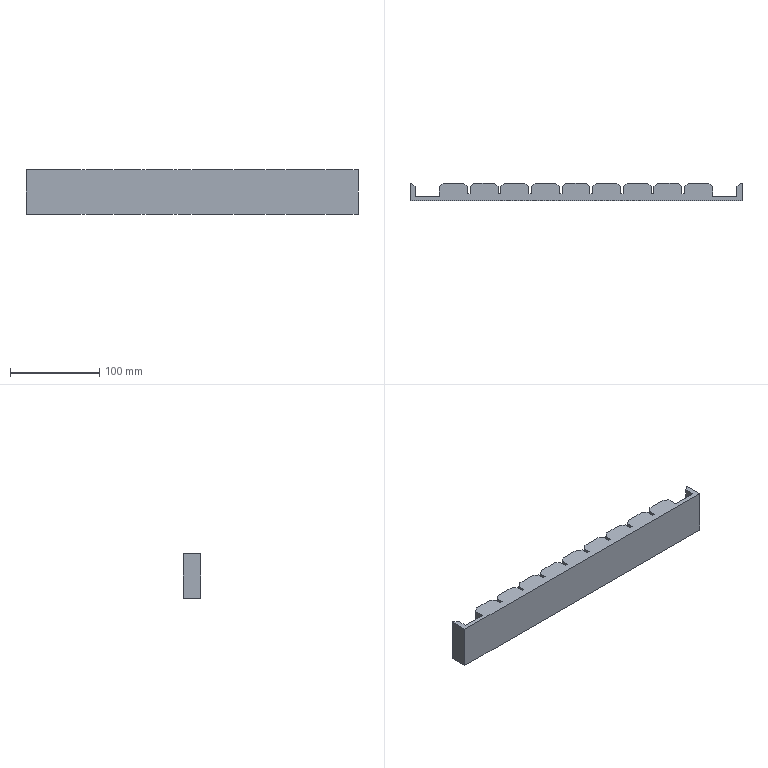NC program | NX | posted with a generic post | part box 372.9 x 20 x 50 mm
Lines 1464 to 3956 of 3956, first 2432 of 2489 lines:
(PLANAR_MILL , TOOL : D3)
N2926 T16 M6
N2928 G17 G43 G0 G90 X-120.54 Y-28. Z30. S9500 H16 M3
N2930 Z2.7
N2932 G94 G1 Z-0.3 F1800.
N2934 Y-25.
N2936 Y25.
N2938 Y28.
N2940 Z2.7
N2942 G0 Y-28. Z2.4
N2944 G1 Z-0.6
N2946 Y-25.
N2948 Y25.
N2950 Y28.
N2952 Z2.4
N2954 G0 Y-28. Z2.1
N2956 G1 Z-0.9
N2958 Y-25.
N2960 Y25.
N2962 Y28.
N2964 Z2.1
N2966 G0 Y-28. Z1.8
N2968 G1 Z-1.2
N2970 Y-25.
N2972 Y25.
N2974 Y28.
N2976 Z1.8
N2978 G0 Y-28. Z1.5
N2980 G1 Z-1.5
N2982 Y-25.
N2984 Y25.
N2986 Y28.
N2988 Z1.5
N2990 G0 Y-28. Z1.2
N2992 G1 Z-1.8
N2994 Y-25.
N2996 Y25.
N2998 Y28.
N3000 Z1.2
N3002 G0 Y-28. Z0.9
N3004 G1 Z-2.1
N3006 Y-25.
N3008 Y25.
N3010 Y28.
N3012 Z0.9
N3014 G0 Y-28. Z0.6
N3016 G1 Z-2.4
N3018 Y-25.
N3020 Y25.
N3022 Y28.
N3024 Z0.6
N3026 G0 Y-28. Z0.3
N3028 G1 Z-2.7
N3030 Y-25.
N3032 Y25.
N3034 Y28.
N3036 Z0.3
N3038 G0 Y-28. Z0.
N3040 G1 Z-3.
N3042 Y-25.
N3044 Y25.
N3046 Y28.
N3048 Z0.
N3050 G0 Y-28. Z-0.3
N3052 G1 Z-3.3
N3054 Y-25.
N3056 Y25.
N3058 Y28.
N3060 Z-0.3
N3062 G0 Y-28. Z-0.6
N3064 G1 Z-3.6
N3066 Y-25.
N3068 Y25.
N3070 Y28.
N3072 Z-0.6
N3074 G0 Y-28. Z-0.9
N3076 G1 Z-3.9
N3078 Y-25.
N3080 Y25.
N3082 Y28.
N3084 Z-0.9
N3086 G0 Y-28. Z-1.2
N3088 G1 Z-4.2
N3090 Y-25.
N3092 Y25.
N3094 Y28.
N3096 Z-1.2
N3098 G0 Y-28. Z-1.5
N3100 G1 Z-4.5
N3102 Y-25.
N3104 Y25.
N3106 Y28.
N3108 Z-1.5
N3110 G0 Y-28. Z-1.8
N3112 G1 Z-4.8
N3114 Y-25.
N3116 Y25.
N3118 Y28.
N3120 Z-1.8
N3122 G0 Y-28. Z-2.1
N3124 G1 Z-5.1
N3126 Y-25.
N3128 Y25.
N3130 Y28.
N3132 Z-2.1
N3134 G0 Y-28. Z-2.4
N3136 G1 Z-5.4
N3138 Y-25.
N3140 Y25.
N3142 Y28.
N3144 Z-2.4
N3146 G0 Y-28. Z-2.7
N3148 G1 Z-5.7
N3150 Y-25.
N3152 Y25.
N3154 Y28.
N3156 Z-2.7
N3158 G0 Y-28. Z-3.
N3160 G1 Z-6.
N3162 Y-25.
N3164 Y25.
N3166 Y28.
N3168 Z-3.
N3170 G0 Y-28. Z-3.3
N3172 G1 Z-6.3
N3174 Y-25.
N3176 Y25.
N3178 Y28.
N3180 Z-3.3
N3182 G0 Y-28. Z-3.6
N3184 G1 Z-6.6
N3186 Y-25.
N3188 Y25.
N3190 Y28.
N3192 Z-3.6
N3194 G0 Y-28. Z-3.9
N3196 G1 Z-6.9
N3198 Y-25.
N3200 Y25.
N3202 Y28.
N3204 Z-3.9
N3206 G0 Y-28. Z-4.2
N3208 G1 Z-7.2
N3210 Y-25.
N3212 Y25.
N3214 Y28.
N3216 Z-4.2
N3218 G0 Y-28. Z-4.5
N3220 G1 Z-7.5
N3222 Y-25.
N3224 Y25.
N3226 Y28.
N3228 Z-4.5
N3230 G0 Y-28. Z-4.8
N3232 G1 Z-7.8
N3234 Y-25.
N3236 Y25.
N3238 Y28.
N3240 Z-4.8
N3242 G0 Y-28. Z-5.1
N3244 G1 Z-8.1
N3246 Y-25.
N3248 Y25.
N3250 Y28.
N3252 Z-5.1
N3254 G0 Y-28. Z-5.4
N3256 G1 Z-8.4
N3258 Y-25.
N3260 Y25.
N3262 Y28.
N3264 Z-5.4
N3266 G0 Y-28. Z-5.7
N3268 G1 Z-8.7
N3270 Y-25.
N3272 Y25.
N3274 Y28.
N3276 Z-5.7
N3278 G0 Y-28. Z-6.
N3280 G1 Z-9.
N3282 Y-25.
N3284 Y25.
N3286 Y28.
N3288 Z-6.
N3290 G0 Y-28. Z-6.3
N3292 G1 Z-9.3
N3294 Y-25.
N3296 Y25.
N3298 Y28.
N3300 Z-6.3
N3302 G0 Y-28. Z-6.6
N3304 G1 Z-9.6
N3306 Y-25.
N3308 Y25.
N3310 Y28.
N3312 Z-6.6
N3314 G0 Y-28. Z-6.9
N3316 G1 Z-9.9
N3318 Y-25.
N3320 Y25.
N3322 Y28.
N3324 Z-6.9
N3326 G0 Y-28. Z-7.2
N3328 G1 Z-10.2
N3330 Y-25.
N3332 Y25.
N3334 Y28.
N3336 Z-7.2
N3338 G0 Y-28. Z-7.5
N3340 G1 Z-10.5
N3342 Y-25.
N3344 Y25.
N3346 Y28.
N3348 Z-7.5
N3350 G0 Y-28. Z-7.8
N3352 G1 Z-10.8
N3354 Y-25.
N3356 Y25.
N3358 Y28.
N3360 Z-7.8
N3362 G0 Y-28. Z-8.1
N3364 G1 Z-11.1
N3366 Y-25.
N3368 Y25.
N3370 Y28.
N3372 Z-8.1
N3374 G0 Y-28. Z-8.4
N3376 G1 Z-11.4
N3378 Y-25.
N3380 Y25.
N3382 Y28.
N3384 Z-8.4
N3386 G0 Y-28. Z-8.7
N3388 G1 Z-11.7
N3390 Y-25.
N3392 Y25.
N3394 Y28.
N3396 Z-8.7
N3398 G0 Y-28. Z-9.
N3400 G1 Z-12.
N3402 Y-25.
N3404 Y25.
N3406 Y28.
N3408 Z-9.
N3410 G0 Z30.
N3412 X-86.1 Y-28.
N3414 Z2.7
N3416 G1 Z-0.3
N3418 Y-25.
N3420 Y25.
N3422 Y28.
N3424 Z2.7
N3426 G0 Y-28. Z2.4
N3428 G1 Z-0.6
N3430 Y-25.
N3432 Y25.
N3434 Y28.
N3436 Z2.4
N3438 G0 Y-28. Z2.1
N3440 G1 Z-0.9
N3442 Y-25.
N3444 Y25.
N3446 Y28.
N3448 Z2.1
N3450 G0 Y-28. Z1.8
N3452 G1 Z-1.2
N3454 Y-25.
N3456 Y25.
N3458 Y28.
N3460 Z1.8
N3462 G0 Y-28. Z1.5
N3464 G1 Z-1.5
N3466 Y-25.
N3468 Y25.
N3470 Y28.
N3472 Z1.5
N3474 G0 Y-28. Z1.2
N3476 G1 Z-1.8
N3478 Y-25.
N3480 Y25.
N3482 Y28.
N3484 Z1.2
N3486 G0 Y-28. Z0.9
N3488 G1 Z-2.1
N3490 Y-25.
N3492 Y25.
N3494 Y28.
N3496 Z0.9
N3498 G0 Y-28. Z0.6
N3500 G1 Z-2.4
N3502 Y-25.
N3504 Y25.
N3506 Y28.
N3508 Z0.6
N3510 G0 Y-28. Z0.3
N3512 G1 Z-2.7
N3514 Y-25.
N3516 Y25.
N3518 Y28.
N3520 Z0.3
N3522 G0 Y-28. Z0.
N3524 G1 Z-3.
N3526 Y-25.
N3528 Y25.
N3530 Y28.
N3532 Z0.
N3534 G0 Y-28. Z-0.3
N3536 G1 Z-3.3
N3538 Y-25.
N3540 Y25.
N3542 Y28.
N3544 Z-0.3
N3546 G0 Y-28. Z-0.6
N3548 G1 Z-3.6
N3550 Y-25.
N3552 Y25.
N3554 Y28.
N3556 Z-0.6
N3558 G0 Y-28. Z-0.9
N3560 G1 Z-3.9
N3562 Y-25.
N3564 Y25.
N3566 Y28.
N3568 Z-0.9
N3570 G0 Y-28. Z-1.2
N3572 G1 Z-4.2
N3574 Y-25.
N3576 Y25.
N3578 Y28.
N3580 Z-1.2
N3582 G0 Y-28. Z-1.5
N3584 G1 Z-4.5
N3586 Y-25.
N3588 Y25.
N3590 Y28.
N3592 Z-1.5
N3594 G0 Y-28. Z-1.8
N3596 G1 Z-4.8
N3598 Y-25.
N3600 Y25.
N3602 Y28.
N3604 Z-1.8
N3606 G0 Y-28. Z-2.1
N3608 G1 Z-5.1
N3610 Y-25.
N3612 Y25.
N3614 Y28.
N3616 Z-2.1
N3618 G0 Y-28. Z-2.4
N3620 G1 Z-5.4
N3622 Y-25.
N3624 Y25.
N3626 Y28.
N3628 Z-2.4
N3630 G0 Y-28. Z-2.7
N3632 G1 Z-5.7
N3634 Y-25.
N3636 Y25.
N3638 Y28.
N3640 Z-2.7
N3642 G0 Y-28. Z-3.
N3644 G1 Z-6.
N3646 Y-25.
N3648 Y25.
N3650 Y28.
N3652 Z-3.
N3654 G0 Y-28. Z-3.3
N3656 G1 Z-6.3
N3658 Y-25.
N3660 Y25.
N3662 Y28.
N3664 Z-3.3
N3666 G0 Y-28. Z-3.6
N3668 G1 Z-6.6
N3670 Y-25.
N3672 Y25.
N3674 Y28.
N3676 Z-3.6
N3678 G0 Y-28. Z-3.9
N3680 G1 Z-6.9
N3682 Y-25.
N3684 Y25.
N3686 Y28.
N3688 Z-3.9
N3690 G0 Y-28. Z-4.2
N3692 G1 Z-7.2
N3694 Y-25.
N3696 Y25.
N3698 Y28.
N3700 Z-4.2
N3702 G0 Y-28. Z-4.5
N3704 G1 Z-7.5
N3706 Y-25.
N3708 Y25.
N3710 Y28.
N3712 Z-4.5
N3714 G0 Y-28. Z-4.8
N3716 G1 Z-7.8
N3718 Y-25.
N3720 Y25.
N3722 Y28.
N3724 Z-4.8
N3726 G0 Y-28. Z-5.1
N3728 G1 Z-8.1
N3730 Y-25.
N3732 Y25.
N3734 Y28.
N3736 Z-5.1
N3738 G0 Y-28. Z-5.4
N3740 G1 Z-8.4
N3742 Y-25.
N3744 Y25.
N3746 Y28.
N3748 Z-5.4
N3750 G0 Y-28. Z-5.7
N3752 G1 Z-8.7
N3754 Y-25.
N3756 Y25.
N3758 Y28.
N3760 Z-5.7
N3762 G0 Y-28. Z-6.
N3764 G1 Z-9.
N3766 Y-25.
N3768 Y25.
N3770 Y28.
N3772 Z-6.
N3774 G0 Y-28. Z-6.3
N3776 G1 Z-9.3
N3778 Y-25.
N3780 Y25.
N3782 Y28.
N3784 Z-6.3
N3786 G0 Y-28. Z-6.6
N3788 G1 Z-9.6
N3790 Y-25.
N3792 Y25.
N3794 Y28.
N3796 Z-6.6
N3798 G0 Y-28. Z-6.9
N3800 G1 Z-9.9
N3802 Y-25.
N3804 Y25.
N3806 Y28.
N3808 Z-6.9
N3810 G0 Y-28. Z-7.2
N3812 G1 Z-10.2
N3814 Y-25.
N3816 Y25.
N3818 Y28.
N3820 Z-7.2
N3822 G0 Y-28. Z-7.5
N3824 G1 Z-10.5
N3826 Y-25.
N3828 Y25.
N3830 Y28.
N3832 Z-7.5
N3834 G0 Y-28. Z-7.8
N3836 G1 Z-10.8
N3838 Y-25.
N3840 Y25.
N3842 Y28.
N3844 Z-7.8
N3846 G0 Y-28. Z-8.1
N3848 G1 Z-11.1
N3850 Y-25.
N3852 Y25.
N3854 Y28.
N3856 Z-8.1
N3858 G0 Y-28. Z-8.4
N3860 G1 Z-11.4
N3862 Y-25.
N3864 Y25.
N3866 Y28.
N3868 Z-8.4
N3870 G0 Y-28. Z-8.7
N3872 G1 Z-11.7
N3874 Y-25.
N3876 Y25.
N3878 Y28.
N3880 Z-8.7
N3882 G0 Y-28. Z-9.
N3884 G1 Z-12.
N3886 Y-25.
N3888 Y25.
N3890 Y28.
N3892 Z-9.
N3894 G0 Z30.
N3896 X-51.66 Y-28.
N3898 Z2.7
N3900 G1 Z-0.3
N3902 Y-25.
N3904 Y25.
N3906 Y28.
N3908 Z2.7
N3910 G0 Y-28. Z2.4
N3912 G1 Z-0.6
N3914 Y-25.
N3916 Y25.
N3918 Y28.
N3920 Z2.4
N3922 G0 Y-28. Z2.1
N3924 G1 Z-0.9
N3926 Y-25.
N3928 Y25.
N3930 Y28.
N3932 Z2.1
N3934 G0 Y-28. Z1.8
N3936 G1 Z-1.2
N3938 Y-25.
N3940 Y25.
N3942 Y28.
N3944 Z1.8
N3946 G0 Y-28. Z1.5
N3948 G1 Z-1.5
N3950 Y-25.
N3952 Y25.
N3954 Y28.
N3956 Z1.5
N3958 G0 Y-28. Z1.2
N3960 G1 Z-1.8
N3962 Y-25.
N3964 Y25.
N3966 Y28.
N3968 Z1.2
N3970 G0 Y-28. Z0.9
N3972 G1 Z-2.1
N3974 Y-25.
N3976 Y25.
N3978 Y28.
N3980 Z0.9
N3982 G0 Y-28. Z0.6
N3984 G1 Z-2.4
N3986 Y-25.
N3988 Y25.
N3990 Y28.
N3992 Z0.6
N3994 G0 Y-28. Z0.3
N3996 G1 Z-2.7
N3998 Y-25.
N4000 Y25.
N4002 Y28.
N4004 Z0.3
N4006 G0 Y-28. Z0.
N4008 G1 Z-3.
N4010 Y-25.
N4012 Y25.
N4014 Y28.
N4016 Z0.
N4018 G0 Y-28. Z-0.3
N4020 G1 Z-3.3
N4022 Y-25.
N4024 Y25.
N4026 Y28.
N4028 Z-0.3
N4030 G0 Y-28. Z-0.6
N4032 G1 Z-3.6
N4034 Y-25.
N4036 Y25.
N4038 Y28.
N4040 Z-0.6
N4042 G0 Y-28. Z-0.9
N4044 G1 Z-3.9
N4046 Y-25.
N4048 Y25.
N4050 Y28.
N4052 Z-0.9
N4054 G0 Y-28. Z-1.2
N4056 G1 Z-4.2
N4058 Y-25.
N4060 Y25.
N4062 Y28.
N4064 Z-1.2
N4066 G0 Y-28. Z-1.5
N4068 G1 Z-4.5
N4070 Y-25.
N4072 Y25.
N4074 Y28.
N4076 Z-1.5
N4078 G0 Y-28. Z-1.8
N4080 G1 Z-4.8
N4082 Y-25.
N4084 Y25.
N4086 Y28.
N4088 Z-1.8
N4090 G0 Y-28. Z-2.1
N4092 G1 Z-5.1
N4094 Y-25.
N4096 Y25.
N4098 Y28.
N4100 Z-2.1
N4102 G0 Y-28. Z-2.4
N4104 G1 Z-5.4
N4106 Y-25.
N4108 Y25.
N4110 Y28.
N4112 Z-2.4
N4114 G0 Y-28. Z-2.7
N4116 G1 Z-5.7
N4118 Y-25.
N4120 Y25.
N4122 Y28.
N4124 Z-2.7
N4126 G0 Y-28. Z-3.
N4128 G1 Z-6.
N4130 Y-25.
N4132 Y25.
N4134 Y28.
N4136 Z-3.
N4138 G0 Y-28. Z-3.3
N4140 G1 Z-6.3
N4142 Y-25.
N4144 Y25.
N4146 Y28.
N4148 Z-3.3
N4150 G0 Y-28. Z-3.6
N4152 G1 Z-6.6
N4154 Y-25.
N4156 Y25.
N4158 Y28.
N4160 Z-3.6
N4162 G0 Y-28. Z-3.9
N4164 G1 Z-6.9
N4166 Y-25.
N4168 Y25.
N4170 Y28.
N4172 Z-3.9
N4174 G0 Y-28. Z-4.2
N4176 G1 Z-7.2
N4178 Y-25.
N4180 Y25.
N4182 Y28.
N4184 Z-4.2
N4186 G0 Y-28. Z-4.5
N4188 G1 Z-7.5
N4190 Y-25.
N4192 Y25.
N4194 Y28.
N4196 Z-4.5
N4198 G0 Y-28. Z-4.8
N4200 G1 Z-7.8
N4202 Y-25.
N4204 Y25.
N4206 Y28.
N4208 Z-4.8
N4210 G0 Y-28. Z-5.1
N4212 G1 Z-8.1
N4214 Y-25.
N4216 Y25.
N4218 Y28.
N4220 Z-5.1
N4222 G0 Y-28. Z-5.4
N4224 G1 Z-8.4
N4226 Y-25.
N4228 Y25.
N4230 Y28.
N4232 Z-5.4
N4234 G0 Y-28. Z-5.7
N4236 G1 Z-8.7
N4238 Y-25.
N4240 Y25.
N4242 Y28.
N4244 Z-5.7
N4246 G0 Y-28. Z-6.
N4248 G1 Z-9.
N4250 Y-25.
N4252 Y25.
N4254 Y28.
N4256 Z-6.
N4258 G0 Y-28. Z-6.3
N4260 G1 Z-9.3
N4262 Y-25.
N4264 Y25.
N4266 Y28.
N4268 Z-6.3
N4270 G0 Y-28. Z-6.6
N4272 G1 Z-9.6
N4274 Y-25.
N4276 Y25.
N4278 Y28.
N4280 Z-6.6
N4282 G0 Y-28. Z-6.9
N4284 G1 Z-9.9
N4286 Y-25.
N4288 Y25.
N4290 Y28.
N4292 Z-6.9
N4294 G0 Y-28. Z-7.2
N4296 G1 Z-10.2
N4298 Y-25.
N4300 Y25.
N4302 Y28.
N4304 Z-7.2
N4306 G0 Y-28. Z-7.5
N4308 G1 Z-10.5
N4310 Y-25.
N4312 Y25.
N4314 Y28.
N4316 Z-7.5
N4318 G0 Y-28. Z-7.8
N4320 G1 Z-10.8
N4322 Y-25.
N4324 Y25.
N4326 Y28.
N4328 Z-7.8
N4330 G0 Y-28. Z-8.1
N4332 G1 Z-11.1
N4334 Y-25.
N4336 Y25.
N4338 Y28.
N4340 Z-8.1
N4342 G0 Y-28. Z-8.4
N4344 G1 Z-11.4
N4346 Y-25.
N4348 Y25.
N4350 Y28.
N4352 Z-8.4
N4354 G0 Y-28. Z-8.7
N4356 G1 Z-11.7
N4358 Y-25.
N4360 Y25.
N4362 Y28.
N4364 Z-8.7
N4366 G0 Y-28. Z-9.
N4368 G1 Z-12.
N4370 Y-25.
N4372 Y25.
N4374 Y28.
N4376 Z-9.
N4378 G0 Z30.
N4380 X-17.22 Y-28.
N4382 Z2.7
N4384 G1 Z-0.3
N4386 Y-25.
N4388 Y25.
N4390 Y28.
N4392 Z2.7
N4394 G0 Y-28. Z2.4
N4396 G1 Z-0.6
N4398 Y-25.
N4400 Y25.
N4402 Y28.
N4404 Z2.4
N4406 G0 Y-28. Z2.1
N4408 G1 Z-0.9
N4410 Y-25.
N4412 Y25.
N4414 Y28.
N4416 Z2.1
N4418 G0 Y-28. Z1.8
N4420 G1 Z-1.2
N4422 Y-25.
N4424 Y25.
N4426 Y28.
N4428 Z1.8
N4430 G0 Y-28. Z1.5
N4432 G1 Z-1.5
N4434 Y-25.
N4436 Y25.
N4438 Y28.
N4440 Z1.5
N4442 G0 Y-28. Z1.2
N4444 G1 Z-1.8
N4446 Y-25.
N4448 Y25.
N4450 Y28.
N4452 Z1.2
N4454 G0 Y-28. Z0.9
N4456 G1 Z-2.1
N4458 Y-25.
N4460 Y25.
N4462 Y28.
N4464 Z0.9
N4466 G0 Y-28. Z0.6
N4468 G1 Z-2.4
N4470 Y-25.
N4472 Y25.
N4474 Y28.
N4476 Z0.6
N4478 G0 Y-28. Z0.3
N4480 G1 Z-2.7
N4482 Y-25.
N4484 Y25.
N4486 Y28.
N4488 Z0.3
N4490 G0 Y-28. Z0.
N4492 G1 Z-3.
N4494 Y-25.
N4496 Y25.
N4498 Y28.
N4500 Z0.
N4502 G0 Y-28. Z-0.3
N4504 G1 Z-3.3
N4506 Y-25.
N4508 Y25.
N4510 Y28.
N4512 Z-0.3
N4514 G0 Y-28. Z-0.6
N4516 G1 Z-3.6
N4518 Y-25.
N4520 Y25.
N4522 Y28.
N4524 Z-0.6
N4526 G0 Y-28. Z-0.9
N4528 G1 Z-3.9
N4530 Y-25.
N4532 Y25.
N4534 Y28.
N4536 Z-0.9
N4538 G0 Y-28. Z-1.2
N4540 G1 Z-4.2
N4542 Y-25.
N4544 Y25.
N4546 Y28.
N4548 Z-1.2
N4550 G0 Y-28. Z-1.5
N4552 G1 Z-4.5
N4554 Y-25.
N4556 Y25.
N4558 Y28.
N4560 Z-1.5
N4562 G0 Y-28. Z-1.8
N4564 G1 Z-4.8
N4566 Y-25.
N4568 Y25.
N4570 Y28.
N4572 Z-1.8
N4574 G0 Y-28. Z-2.1
N4576 G1 Z-5.1
N4578 Y-25.
N4580 Y25.
N4582 Y28.
N4584 Z-2.1
N4586 G0 Y-28. Z-2.4
N4588 G1 Z-5.4
N4590 Y-25.
N4592 Y25.
N4594 Y28.
N4596 Z-2.4
N4598 G0 Y-28. Z-2.7
N4600 G1 Z-5.7
N4602 Y-25.
N4604 Y25.
N4606 Y28.
N4608 Z-2.7
N4610 G0 Y-28. Z-3.
N4612 G1 Z-6.
N4614 Y-25.
N4616 Y25.
N4618 Y28.
N4620 Z-3.
N4622 G0 Y-28. Z-3.3
N4624 G1 Z-6.3
N4626 Y-25.
N4628 Y25.
N4630 Y28.
N4632 Z-3.3
N4634 G0 Y-28. Z-3.6
N4636 G1 Z-6.6
N4638 Y-25.
N4640 Y25.
N4642 Y28.
N4644 Z-3.6
N4646 G0 Y-28. Z-3.9
N4648 G1 Z-6.9
N4650 Y-25.
N4652 Y25.
N4654 Y28.
N4656 Z-3.9
N4658 G0 Y-28. Z-4.2
N4660 G1 Z-7.2
N4662 Y-25.
N4664 Y25.
N4666 Y28.
N4668 Z-4.2
N4670 G0 Y-28. Z-4.5
N4672 G1 Z-7.5
N4674 Y-25.
N4676 Y25.
N4678 Y28.
N4680 Z-4.5
N4682 G0 Y-28. Z-4.8
N4684 G1 Z-7.8
N4686 Y-25.
N4688 Y25.
N4690 Y28.
N4692 Z-4.8
N4694 G0 Y-28. Z-5.1
N4696 G1 Z-8.1
N4698 Y-25.
N4700 Y25.
N4702 Y28.
N4704 Z-5.1
N4706 G0 Y-28. Z-5.4
N4708 G1 Z-8.4
N4710 Y-25.
N4712 Y25.
N4714 Y28.
N4716 Z-5.4
N4718 G0 Y-28. Z-5.7
N4720 G1 Z-8.7
N4722 Y-25.
N4724 Y25.
N4726 Y28.
N4728 Z-5.7
N4730 G0 Y-28. Z-6.
N4732 G1 Z-9.
N4734 Y-25.
N4736 Y25.
N4738 Y28.
N4740 Z-6.
N4742 G0 Y-28. Z-6.3
N4744 G1 Z-9.3
N4746 Y-25.
N4748 Y25.
N4750 Y28.
N4752 Z-6.3
N4754 G0 Y-28. Z-6.6
N4756 G1 Z-9.6
N4758 Y-25.
N4760 Y25.
N4762 Y28.
N4764 Z-6.6
N4766 G0 Y-28. Z-6.9
N4768 G1 Z-9.9
N4770 Y-25.
N4772 Y25.
N4774 Y28.
N4776 Z-6.9
N4778 G0 Y-28. Z-7.2
N4780 G1 Z-10.2
N4782 Y-25.
N4784 Y25.
N4786 Y28.
N4788 Z-7.2
N4790 G0 Y-28. Z-7.5
N4792 G1 Z-10.5
N4794 Y-25.
N4796 Y25.
N4798 Y28.
N4800 Z-7.5
N4802 G0 Y-28. Z-7.8
N4804 G1 Z-10.8
N4806 Y-25.
N4808 Y25.
N4810 Y28.
N4812 Z-7.8
N4814 G0 Y-28. Z-8.1
N4816 G1 Z-11.1
N4818 Y-25.
N4820 Y25.
N4822 Y28.
N4824 Z-8.1
N4826 G0 Y-28. Z-8.4
N4828 G1 Z-11.4
N4830 Y-25.
N4832 Y25.
N4834 Y28.
N4836 Z-8.4
N4838 G0 Y-28. Z-8.7
N4840 G1 Z-11.7
N4842 Y-25.
N4844 Y25.
N4846 Y28.
N4848 Z-8.7
N4850 G0 Y-28. Z-9.
N4852 G1 Z-12.
N4854 Y-25.
N4856 Y25.
N4858 Y28.
N4860 Z-9.
N4862 G0 Z30.
N4864 X17.22 Y-28.
N4866 Z2.7
N4868 G1 Z-0.3
N4870 Y-25.
N4872 Y25.
N4874 Y28.
N4876 Z2.7
N4878 G0 Y-28. Z2.4
N4880 G1 Z-0.6
N4882 Y-25.
N4884 Y25.
N4886 Y28.
N4888 Z2.4
N4890 G0 Y-28. Z2.1
N4892 G1 Z-0.9
N4894 Y-25.
N4896 Y25.
N4898 Y28.
N4900 Z2.1
N4902 G0 Y-28. Z1.8
N4904 G1 Z-1.2
N4906 Y-25.
N4908 Y25.
N4910 Y28.
N4912 Z1.8
N4914 G0 Y-28. Z1.5
N4916 G1 Z-1.5
N4918 Y-25.
N4920 Y25.
N4922 Y28.
N4924 Z1.5
N4926 G0 Y-28. Z1.2
N4928 G1 Z-1.8
N4930 Y-25.
N4932 Y25.
N4934 Y28.
N4936 Z1.2
N4938 G0 Y-28. Z0.9
N4940 G1 Z-2.1
N4942 Y-25.
N4944 Y25.
N4946 Y28.
N4948 Z0.9
N4950 G0 Y-28. Z0.6
N4952 G1 Z-2.4
N4954 Y-25.
N4956 Y25.
N4958 Y28.
N4960 Z0.6
N4962 G0 Y-28. Z0.3
N4964 G1 Z-2.7
N4966 Y-25.
N4968 Y25.
N4970 Y28.
N4972 Z0.3
N4974 G0 Y-28. Z0.
N4976 G1 Z-3.
N4978 Y-25.
N4980 Y25.
N4982 Y28.
N4984 Z0.
N4986 G0 Y-28. Z-0.3
N4988 G1 Z-3.3
N4990 Y-25.
N4992 Y25.
N4994 Y28.
N4996 Z-0.3
N4998 G0 Y-28. Z-0.6
N5000 G1 Z-3.6
N5002 Y-25.
N5004 Y25.
N5006 Y28.
N5008 Z-0.6
N5010 G0 Y-28. Z-0.9
N5012 G1 Z-3.9
N5014 Y-25.
N5016 Y25.
N5018 Y28.
N5020 Z-0.9
N5022 G0 Y-28. Z-1.2
N5024 G1 Z-4.2
N5026 Y-25.
N5028 Y25.
N5030 Y28.
N5032 Z-1.2
N5034 G0 Y-28. Z-1.5
N5036 G1 Z-4.5
N5038 Y-25.
N5040 Y25.
N5042 Y28.
N5044 Z-1.5
N5046 G0 Y-28. Z-1.8
N5048 G1 Z-4.8
N5050 Y-25.
N5052 Y25.
N5054 Y28.
N5056 Z-1.8
N5058 G0 Y-28. Z-2.1
N5060 G1 Z-5.1
N5062 Y-25.
N5064 Y25.
N5066 Y28.
N5068 Z-2.1
N5070 G0 Y-28. Z-2.4
N5072 G1 Z-5.4
N5074 Y-25.
N5076 Y25.
N5078 Y28.
N5080 Z-2.4
N5082 G0 Y-28. Z-2.7
N5084 G1 Z-5.7
N5086 Y-25.
N5088 Y25.
N5090 Y28.
N5092 Z-2.7
N5094 G0 Y-28. Z-3.
N5096 G1 Z-6.
N5098 Y-25.
N5100 Y25.
N5102 Y28.
N5104 Z-3.
N5106 G0 Y-28. Z-3.3
N5108 G1 Z-6.3
N5110 Y-25.
N5112 Y25.
N5114 Y28.
N5116 Z-3.3
N5118 G0 Y-28. Z-3.6
N5120 G1 Z-6.6
N5122 Y-25.
N5124 Y25.
N5126 Y28.
N5128 Z-3.6
N5130 G0 Y-28. Z-3.9
N5132 G1 Z-6.9
N5134 Y-25.
N5136 Y25.
N5138 Y28.
N5140 Z-3.9
N5142 G0 Y-28. Z-4.2
N5144 G1 Z-7.2
N5146 Y-25.
N5148 Y25.
N5150 Y28.
N5152 Z-4.2
N5154 G0 Y-28. Z-4.5
N5156 G1 Z-7.5
N5158 Y-25.
N5160 Y25.
N5162 Y28.
N5164 Z-4.5
N5166 G0 Y-28. Z-4.8
N5168 G1 Z-7.8
N5170 Y-25.
N5172 Y25.
N5174 Y28.
N5176 Z-4.8
N5178 G0 Y-28. Z-5.1
N5180 G1 Z-8.1
N5182 Y-25.
N5184 Y25.
N5186 Y28.
N5188 Z-5.1
N5190 G0 Y-28. Z-5.4
N5192 G1 Z-8.4
N5194 Y-25.
N5196 Y25.
N5198 Y28.
N5200 Z-5.4
N5202 G0 Y-28. Z-5.7
N5204 G1 Z-8.7
N5206 Y-25.
N5208 Y25.
N5210 Y28.
N5212 Z-5.7
N5214 G0 Y-28. Z-6.
N5216 G1 Z-9.
N5218 Y-25.
N5220 Y25.
N5222 Y28.
N5224 Z-6.
N5226 G0 Y-28. Z-6.3
N5228 G1 Z-9.3
N5230 Y-25.
N5232 Y25.
N5234 Y28.
N5236 Z-6.3
N5238 G0 Y-28. Z-6.6
N5240 G1 Z-9.6
N5242 Y-25.
N5244 Y25.
N5246 Y28.
N5248 Z-6.6
N5250 G0 Y-28. Z-6.9
N5252 G1 Z-9.9
N5254 Y-25.
N5256 Y25.
N5258 Y28.
N5260 Z-6.9
N5262 G0 Y-28. Z-7.2
N5264 G1 Z-10.2
N5266 Y-25.
N5268 Y25.
N5270 Y28.
N5272 Z-7.2
N5274 G0 Y-28. Z-7.5
N5276 G1 Z-10.5
N5278 Y-25.
N5280 Y25.
N5282 Y28.
N5284 Z-7.5
N5286 G0 Y-28. Z-7.8
N5288 G1 Z-10.8
N5290 Y-25.
N5292 Y25.
N5294 Y28.
N5296 Z-7.8
N5298 G0 Y-28. Z-8.1
N5300 G1 Z-11.1
N5302 Y-25.
N5304 Y25.
N5306 Y28.
N5308 Z-8.1
N5310 G0 Y-28. Z-8.4
N5312 G1 Z-11.4
N5314 Y-25.
N5316 Y25.
N5318 Y28.
N5320 Z-8.4
N5322 G0 Y-28. Z-8.7
N5324 G1 Z-11.7
N5326 Y-25.
N5328 Y25.
N5330 Y28.
N5332 Z-8.7
N5334 G0 Y-28. Z-9.
N5336 G1 Z-12.
N5338 Y-25.
N5340 Y25.
N5342 Y28.
N5344 Z-9.
N5346 G0 Z30.
N5348 X51.66 Y-28.
N5350 Z2.7
N5352 G1 Z-0.3
N5354 Y-25.
N5356 Y25.
N5358 Y28.
N5360 Z2.7
N5362 G0 Y-28. Z2.4
N5364 G1 Z-0.6
N5366 Y-25.
N5368 Y25.
N5370 Y28.
N5372 Z2.4
N5374 G0 Y-28. Z2.1
N5376 G1 Z-0.9
N5378 Y-25.
N5380 Y25.
N5382 Y28.
N5384 Z2.1
N5386 G0 Y-28. Z1.8
N5388 G1 Z-1.2
N5390 Y-25.
N5392 Y25.
N5394 Y28.
N5396 Z1.8
N5398 G0 Y-28. Z1.5
N5400 G1 Z-1.5
N5402 Y-25.
N5404 Y25.
N5406 Y28.
N5408 Z1.5
N5410 G0 Y-28. Z1.2
N5412 G1 Z-1.8
N5414 Y-25.
N5416 Y25.
N5418 Y28.
N5420 Z1.2
N5422 G0 Y-28. Z0.9
N5424 G1 Z-2.1
N5426 Y-25.
N5428 Y25.
N5430 Y28.
N5432 Z0.9
N5434 G0 Y-28. Z0.6
N5436 G1 Z-2.4
N5438 Y-25.
N5440 Y25.
N5442 Y28.
N5444 Z0.6
N5446 G0 Y-28. Z0.3
N5448 G1 Z-2.7
N5450 Y-25.
N5452 Y25.
N5454 Y28.
N5456 Z0.3
N5458 G0 Y-28. Z0.
N5460 G1 Z-3.
N5462 Y-25.
N5464 Y25.
N5466 Y28.
N5468 Z0.
N5470 G0 Y-28. Z-0.3
N5472 G1 Z-3.3
N5474 Y-25.
N5476 Y25.
N5478 Y28.
N5480 Z-0.3
N5482 G0 Y-28. Z-0.6
N5484 G1 Z-3.6
N5486 Y-25.
N5488 Y25.
N5490 Y28.
N5492 Z-0.6
N5494 G0 Y-28. Z-0.9
N5496 G1 Z-3.9
N5498 Y-25.
N5500 Y25.
N5502 Y28.
N5504 Z-0.9
N5506 G0 Y-28. Z-1.2
N5508 G1 Z-4.2
N5510 Y-25.
N5512 Y25.
N5514 Y28.
N5516 Z-1.2
N5518 G0 Y-28. Z-1.5
N5520 G1 Z-4.5
N5522 Y-25.
N5524 Y25.
N5526 Y28.
N5528 Z-1.5
N5530 G0 Y-28. Z-1.8
N5532 G1 Z-4.8
N5534 Y-25.
N5536 Y25.
N5538 Y28.
N5540 Z-1.8
N5542 G0 Y-28. Z-2.1
N5544 G1 Z-5.1
N5546 Y-25.
N5548 Y25.
N5550 Y28.
N5552 Z-2.1
N5554 G0 Y-28. Z-2.4
N5556 G1 Z-5.4
N5558 Y-25.
N5560 Y25.
N5562 Y28.
N5564 Z-2.4
N5566 G0 Y-28. Z-2.7
N5568 G1 Z-5.7
N5570 Y-25.
N5572 Y25.
N5574 Y28.
N5576 Z-2.7
N5578 G0 Y-28. Z-3.
N5580 G1 Z-6.
N5582 Y-25.
N5584 Y25.
N5586 Y28.
N5588 Z-3.
N5590 G0 Y-28. Z-3.3
N5592 G1 Z-6.3
N5594 Y-25.
N5596 Y25.
N5598 Y28.
N5600 Z-3.3
N5602 G0 Y-28. Z-3.6
N5604 G1 Z-6.6
N5606 Y-25.
N5608 Y25.
N5610 Y28.
N5612 Z-3.6
N5614 G0 Y-28. Z-3.9
N5616 G1 Z-6.9
N5618 Y-25.
N5620 Y25.
N5622 Y28.
N5624 Z-3.9
N5626 G0 Y-28. Z-4.2
N5628 G1 Z-7.2
N5630 Y-25.
N5632 Y25.
N5634 Y28.
N5636 Z-4.2
N5638 G0 Y-28. Z-4.5
N5640 G1 Z-7.5
N5642 Y-25.
N5644 Y25.
N5646 Y28.
N5648 Z-4.5
N5650 G0 Y-28. Z-4.8
N5652 G1 Z-7.8
N5654 Y-25.
N5656 Y25.
N5658 Y28.
N5660 Z-4.8
N5662 G0 Y-28. Z-5.1
N5664 G1 Z-8.1
N5666 Y-25.
N5668 Y25.
N5670 Y28.
N5672 Z-5.1
N5674 G0 Y-28. Z-5.4
N5676 G1 Z-8.4
N5678 Y-25.
N5680 Y25.
N5682 Y28.
N5684 Z-5.4
N5686 G0 Y-28. Z-5.7
N5688 G1 Z-8.7
N5690 Y-25.
N5692 Y25.
N5694 Y28.
N5696 Z-5.7
N5698 G0 Y-28. Z-6.
N5700 G1 Z-9.
N5702 Y-25.
N5704 Y25.
N5706 Y28.
N5708 Z-6.
N5710 G0 Y-28. Z-6.3
N5712 G1 Z-9.3
N5714 Y-25.
N5716 Y25.
N5718 Y28.
N5720 Z-6.3
N5722 G0 Y-28. Z-6.6
N5724 G1 Z-9.6
N5726 Y-25.
N5728 Y25.
N5730 Y28.
N5732 Z-6.6
N5734 G0 Y-28. Z-6.9
N5736 G1 Z-9.9
N5738 Y-25.
N5740 Y25.
N5742 Y28.
N5744 Z-6.9
N5746 G0 Y-28. Z-7.2
N5748 G1 Z-10.2
N5750 Y-25.
N5752 Y25.
N5754 Y28.
N5756 Z-7.2
N5758 G0 Y-28. Z-7.5
N5760 G1 Z-10.5
N5762 Y-25.
N5764 Y25.
N5766 Y28.
N5768 Z-7.5
N5770 G0 Y-28. Z-7.8
N5772 G1 Z-10.8
N5774 Y-25.
N5776 Y25.
N5778 Y28.
N5780 Z-7.8
N5782 G0 Y-28. Z-8.1
N5784 G1 Z-11.1
N5786 Y-25.
N5788 Y25.
N5790 Y28.
N5792 Z-8.1
N5794 G0 Y-28. Z-8.4
N5796 G1 Z-11.4
N5798 Y-25.
N5800 Y25.
N5802 Y28.
N5804 Z-8.4
N5806 G0 Y-28. Z-8.7
N5808 G1 Z-11.7
N5810 Y-25.
N5812 Y25.
N5814 Y28.
N5816 Z-8.7
N5818 G0 Y-28. Z-9.
N5820 G1 Z-12.
N5822 Y-25.
N5824 Y25.
N5826 Y28.
N5828 Z-9.
N5830 G0 Z30.
N5832 X86.1 Y-28.
N5834 Z2.7
N5836 G1 Z-0.3
N5838 Y-25.
N5840 Y25.
N5842 Y28.
N5844 Z2.7
N5846 G0 Y-28. Z2.4
N5848 G1 Z-0.6
N5850 Y-25.
N5852 Y25.
N5854 Y28.
N5856 Z2.4
N5858 G0 Y-28. Z2.1
N5860 G1 Z-0.9
N5862 Y-25.
N5864 Y25.
N5866 Y28.
N5868 Z2.1
N5870 G0 Y-28. Z1.8
N5872 G1 Z-1.2
N5874 Y-25.
N5876 Y25.
N5878 Y28.
N5880 Z1.8
N5882 G0 Y-28. Z1.5
N5884 G1 Z-1.5
N5886 Y-25.
N5888 Y25.
N5890 Y28.
N5892 Z1.5
N5894 G0 Y-28. Z1.2
N5896 G1 Z-1.8
N5898 Y-25.
N5900 Y25.
N5902 Y28.
N5904 Z1.2
N5906 G0 Y-28. Z0.9
N5908 G1 Z-2.1
N5910 Y-25.
N5912 Y25.
N5914 Y28.
N5916 Z0.9
N5918 G0 Y-28. Z0.6
N5920 G1 Z-2.4
N5922 Y-25.
N5924 Y25.
N5926 Y28.
N5928 Z0.6
N5930 G0 Y-28. Z0.3
N5932 G1 Z-2.7
N5934 Y-25.
N5936 Y25.
N5938 Y28.
N5940 Z0.3
N5942 G0 Y-28. Z0.
N5944 G1 Z-3.
N5946 Y-25.
N5948 Y25.
N5950 Y28.
N5952 Z0.
N5954 G0 Y-28. Z-0.3
N5956 G1 Z-3.3
N5958 Y-25.
N5960 Y25.
N5962 Y28.
N5964 Z-0.3
N5966 G0 Y-28. Z-0.6
N5968 G1 Z-3.6
N5970 Y-25.
N5972 Y25.
N5974 Y28.
N5976 Z-0.6
N5978 G0 Y-28. Z-0.9
N5980 G1 Z-3.9
N5982 Y-25.
N5984 Y25.
N5986 Y28.
N5988 Z-0.9
N5990 G0 Y-28. Z-1.2
N5992 G1 Z-4.2
N5994 Y-25.
N5996 Y25.
N5998 Y28.
N6000 Z-1.2
N6002 G0 Y-28. Z-1.5
N6004 G1 Z-4.5
N6006 Y-25.
N6008 Y25.
N6010 Y28.
N6012 Z-1.5
N6014 G0 Y-28. Z-1.8
N6016 G1 Z-4.8
N6018 Y-25.
N6020 Y25.
N6022 Y28.
N6024 Z-1.8
N6026 G0 Y-28. Z-2.1
N6028 G1 Z-5.1
N6030 Y-25.
N6032 Y25.
N6034 Y28.
N6036 Z-2.1
N6038 G0 Y-28. Z-2.4
N6040 G1 Z-5.4
N6042 Y-25.
N6044 Y25.
N6046 Y28.
N6048 Z-2.4
N6050 G0 Y-28. Z-2.7
N6052 G1 Z-5.7
N6054 Y-25.
N6056 Y25.
N6058 Y28.
N6060 Z-2.7
N6062 G0 Y-28. Z-3.
N6064 G1 Z-6.
N6066 Y-25.
N6068 Y25.
N6070 Y28.
N6072 Z-3.
N6074 G0 Y-28. Z-3.3
N6076 G1 Z-6.3
N6078 Y-25.
N6080 Y25.
N6082 Y28.
N6084 Z-3.3
N6086 G0 Y-28. Z-3.6
N6088 G1 Z-6.6
N6090 Y-25.
N6092 Y25.
N6094 Y28.
N6096 Z-3.6
N6098 G0 Y-28. Z-3.9
N6100 G1 Z-6.9
N6102 Y-25.
N6104 Y25.
N6106 Y28.
N6108 Z-3.9
N6110 G0 Y-28. Z-4.2
N6112 G1 Z-7.2
N6114 Y-25.
N6116 Y25.
N6118 Y28.
N6120 Z-4.2
N6122 G0 Y-28. Z-4.5
N6124 G1 Z-7.5
N6126 Y-25.
N6128 Y25.
N6130 Y28.
N6132 Z-4.5
N6134 G0 Y-28. Z-4.8
N6136 G1 Z-7.8
N6138 Y-25.
N6140 Y25.
N6142 Y28.
N6144 Z-4.8
N6146 G0 Y-28. Z-5.1
N6148 G1 Z-8.1
N6150 Y-25.
N6152 Y25.
N6154 Y28.
N6156 Z-5.1
N6158 G0 Y-28. Z-5.4
N6160 G1 Z-8.4
N6162 Y-25.
N6164 Y25.
N6166 Y28.
N6168 Z-5.4
N6170 G0 Y-28. Z-5.7
N6172 G1 Z-8.7
N6174 Y-25.
N6176 Y25.
N6178 Y28.
N6180 Z-5.7
N6182 G0 Y-28. Z-6.
N6184 G1 Z-9.
N6186 Y-25.
N6188 Y25.
N6190 Y28.
N6192 Z-6.
N6194 G0 Y-28. Z-6.3
N6196 G1 Z-9.3
N6198 Y-25.
N6200 Y25.
N6202 Y28.
N6204 Z-6.3
N6206 G0 Y-28. Z-6.6
N6208 G1 Z-9.6
N6210 Y-25.
N6212 Y25.
N6214 Y28.
N6216 Z-6.6
N6218 G0 Y-28. Z-6.9
N6220 G1 Z-9.9
N6222 Y-25.
N6224 Y25.
N6226 Y28.
N6228 Z-6.9
N6230 G0 Y-28. Z-7.2
N6232 G1 Z-10.2
N6234 Y-25.
N6236 Y25.
N6238 Y28.
N6240 Z-7.2
N6242 G0 Y-28. Z-7.5
N6244 G1 Z-10.5
N6246 Y-25.
N6248 Y25.
N6250 Y28.
N6252 Z-7.5
N6254 G0 Y-28. Z-7.8
N6256 G1 Z-10.8
N6258 Y-25.
N6260 Y25.
N6262 Y28.
N6264 Z-7.8
N6266 G0 Y-28. Z-8.1
N6268 G1 Z-11.1
N6270 Y-25.
N6272 Y25.
N6274 Y28.
N6276 Z-8.1
N6278 G0 Y-28. Z-8.4
N6280 G1 Z-11.4
N6282 Y-25.
N6284 Y25.
N6286 Y28.
N6288 Z-8.4
N6290 G0 Y-28. Z-8.7
N6292 G1 Z-11.7
N6294 Y-25.
N6296 Y25.
N6298 Y28.
N6300 Z-8.7
N6302 G0 Y-28. Z-9.
N6304 G1 Z-12.
N6306 Y-25.
N6308 Y25.
N6310 Y28.
N6312 Z-9.
N6314 G0 Z30.
N6316 X120.54 Y-28.
N6318 Z2.7
N6320 G1 Z-0.3
N6322 Y-25.
N6324 Y25.
N6326 Y28.
N6328 Z2.7
N6330 G0 Y-28. Z2.4
N6332 G1 Z-0.6
N6334 Y-25.
N6336 Y25.
N6338 Y28.
N6340 Z2.4
N6342 G0 Y-28. Z2.1
N6344 G1 Z-0.9
N6346 Y-25.
N6348 Y25.
N6350 Y28.
N6352 Z2.1
N6354 G0 Y-28. Z1.8
N6356 G1 Z-1.2
N6358 Y-25.
N6360 Y25.
N6362 Y28.
N6364 Z1.8
N6366 G0 Y-28. Z1.5
N6368 G1 Z-1.5
N6370 Y-25.
N6372 Y25.
N6374 Y28.
N6376 Z1.5
N6378 G0 Y-28. Z1.2
N6380 G1 Z-1.8
N6382 Y-25.
N6384 Y25.
N6386 Y28.
N6388 Z1.2
N6390 G0 Y-28. Z0.9
N6392 G1 Z-2.1
N6394 Y-25.
N6396 Y25.
N6398 Y28.
N6400 Z0.9
N6402 G0 Y-28. Z0.6
N6404 G1 Z-2.4
N6406 Y-25.
N6408 Y25.
N6410 Y28.
N6412 Z0.6
N6414 G0 Y-28. Z0.3
N6416 G1 Z-2.7
N6418 Y-25.
N6420 Y25.
N6422 Y28.
N6424 Z0.3
N6426 G0 Y-28. Z0.
N6428 G1 Z-3.
N6430 Y-25.
N6432 Y25.
N6434 Y28.
N6436 Z0.
N6438 G0 Y-28. Z-0.3
N6440 G1 Z-3.3
N6442 Y-25.
N6444 Y25.
N6446 Y28.
N6448 Z-0.3
N6450 G0 Y-28. Z-0.6
N6452 G1 Z-3.6
N6454 Y-25.
N6456 Y25.
N6458 Y28.
N6460 Z-0.6
N6462 G0 Y-28. Z-0.9
N6464 G1 Z-3.9
N6466 Y-25.
N6468 Y25.
N6470 Y28.
N6472 Z-0.9
N6474 G0 Y-28. Z-1.2
N6476 G1 Z-4.2
N6478 Y-25.
N6480 Y25.
N6482 Y28.
N6484 Z-1.2
N6486 G0 Y-28. Z-1.5
N6488 G1 Z-4.5
N6490 Y-25.
N6492 Y25.
N6494 Y28.
N6496 Z-1.5
N6498 G0 Y-28. Z-1.8
N6500 G1 Z-4.8
N6502 Y-25.
N6504 Y25.
N6506 Y28.
N6508 Z-1.8
N6510 G0 Y-28. Z-2.1
N6512 G1 Z-5.1
N6514 Y-25.
N6516 Y25.
N6518 Y28.
N6520 Z-2.1
N6522 G0 Y-28. Z-2.4
N6524 G1 Z-5.4
N6526 Y-25.
N6528 Y25.
N6530 Y28.
N6532 Z-2.4
N6534 G0 Y-28. Z-2.7
N6536 G1 Z-5.7
N6538 Y-25.
N6540 Y25.
N6542 Y28.
N6544 Z-2.7
N6546 G0 Y-28. Z-3.
N6548 G1 Z-6.
N6550 Y-25.
N6552 Y25.
N6554 Y28.
N6556 Z-3.
N6558 G0 Y-28. Z-3.3
N6560 G1 Z-6.3
N6562 Y-25.
N6564 Y25.
N6566 Y28.
N6568 Z-3.3
N6570 G0 Y-28. Z-3.6
N6572 G1 Z-6.6
N6574 Y-25.
N6576 Y25.
N6578 Y28.
N6580 Z-3.6
N6582 G0 Y-28. Z-3.9
N6584 G1 Z-6.9
N6586 Y-25.
N6588 Y25.
N6590 Y28.
N6592 Z-3.9
N6594 G0 Y-28. Z-4.2
N6596 G1 Z-7.2
N6598 Y-25.
N6600 Y25.
N6602 Y28.
N6604 Z-4.2
N6606 G0 Y-28. Z-4.5
N6608 G1 Z-7.5
N6610 Y-25.
N6612 Y25.
N6614 Y28.
N6616 Z-4.5
N6618 G0 Y-28. Z-4.8
N6620 G1 Z-7.8
N6622 Y-25.
N6624 Y25.
N6626 Y28.
N6628 Z-4.8
N6630 G0 Y-28. Z-5.1
N6632 G1 Z-8.1
N6634 Y-25.
N6636 Y25.
N6638 Y28.
N6640 Z-5.1
N6642 G0 Y-28. Z-5.4
N6644 G1 Z-8.4
N6646 Y-25.
N6648 Y25.
N6650 Y28.
N6652 Z-5.4
N6654 G0 Y-28. Z-5.7
N6656 G1 Z-8.7
N6658 Y-25.
N6660 Y25.
N6662 Y28.
N6664 Z-5.7
N6666 G0 Y-28. Z-6.
N6668 G1 Z-9.
N6670 Y-25.
N6672 Y25.
N6674 Y28.
N6676 Z-6.
N6678 G0 Y-28. Z-6.3
N6680 G1 Z-9.3
N6682 Y-25.
N6684 Y25.
N6686 Y28.
N6688 Z-6.3
N6690 G0 Y-28. Z-6.6
N6692 G1 Z-9.6
N6694 Y-25.
N6696 Y25.
N6698 Y28.
N6700 Z-6.6
N6702 G0 Y-28. Z-6.9
N6704 G1 Z-9.9
N6706 Y-25.
N6708 Y25.
N6710 Y28.
N6712 Z-6.9
N6714 G0 Y-28. Z-7.2
N6716 G1 Z-10.2
N6718 Y-25.
N6720 Y25.
N6722 Y28.
N6724 Z-7.2
N6726 G0 Y-28. Z-7.5
N6728 G1 Z-10.5
N6730 Y-25.
N6732 Y25.
N6734 Y28.
N6736 Z-7.5
N6738 G0 Y-28. Z-7.8
N6740 G1 Z-10.8
N6742 Y-25.
N6744 Y25.
N6746 Y28.
N6748 Z-7.8
N6750 G0 Y-28. Z-8.1
N6752 G1 Z-11.1
N6754 Y-25.
N6756 Y25.
N6758 Y28.
N6760 Z-8.1
N6762 G0 Y-28. Z-8.4
N6764 G1 Z-11.4
N6766 Y-25.
N6768 Y25.
N6770 Y28.
N6772 Z-8.4
N6774 G0 Y-28. Z-8.7
N6776 G1 Z-11.7
N6778 Y-25.
N6780 Y25.
N6782 Y28.
N6784 Z-8.7
N6786 G0 Y-28. Z-9.
N6788 G1 Z-12.
N6790 Y-25.
N6792 Y25.
N6794 Y28.
N6796 Z-9.
N6798 G0 Z30.
N6800 M5
(FLOOR_WALL_1 , TOOL : D6)
N6802 T12 M6
N6804 G54
N6806 G17 G0 G90 X191.35 Y31.118 S9500 M3
N6808 G43 Z30. H12
N6810 Z2.412
N6812 G94 G1 Z-0.588 F850.
N6814 G3 X189.55 Y28. R3.6
N6816 G1 Y-28. F2500.
N6818 G3 X191.35 Y-31.118 R3.6
N6820 G1 Z2.412
N6822 G0 Z3.
N6824 Y31.118
N6826 Z1.824
N6828 G1 Z-1.176 F850.
N6830 G3 X189.55 Y28. R3.6
N6832 G1 Y-28. F2500.
N6834 G3 X191.35 Y-31.118 R3.6
N6836 G1 Z1.824
N6838 G0 Z2.412
N6840 Y31.118
N6842 Z1.235
N6844 G1 Z-1.765 F850.
N6846 G3 X189.55 Y28. R3.6
N6848 G1 Y-28. F2500.
N6850 G3 X191.35 Y-31.118 R3.6
N6852 G1 Z1.235
N6854 G0 Z1.824
N6856 Y31.118
N6858 Z0.647
N6860 G1 Z-2.353 F850.
N6862 G3 X189.55 Y28. R3.6
N6864 G1 Y-28. F2500.
N6866 G3 X191.35 Y-31.118 R3.6
N6868 G1 Z0.647
N6870 G0 Z1.235
N6872 Y31.118
N6874 Z0.059
N6876 G1 Z-2.941 F850.
N6878 G3 X189.55 Y28. R3.6
N6880 G1 Y-28. F2500.
N6882 G3 X191.35 Y-31.118 R3.6
N6884 G1 Z0.059
N6886 G0 Z0.647
N6888 Y31.118
N6890 Z-0.529
N6892 G1 Z-3.529 F850.
N6894 G3 X189.55 Y28. R3.6
N6896 G1 Y-28. F2500.
N6898 G3 X191.35 Y-31.118 R3.6
N6900 G1 Z-0.529
N6902 G0 Z0.059
N6904 Y31.118
N6906 Z-1.118
N6908 G1 Z-4.118 F850.
N6910 G3 X189.55 Y28. R3.6
N6912 G1 Y-28. F2500.
N6914 G3 X191.35 Y-31.118 R3.6
N6916 G1 Z-1.118
N6918 G0 Z-0.529
N6920 Y31.118
N6922 Z-1.706
N6924 G1 Z-4.706 F850.
N6926 G3 X189.55 Y28. R3.6
N6928 G1 Y-28. F2500.
N6930 G3 X191.35 Y-31.118 R3.6
N6932 G1 Z-1.706
N6934 G0 Z-1.118
N6936 Y31.118
N6938 Z-2.294
N6940 G1 Z-5.294 F850.
N6942 G3 X189.55 Y28. R3.6
N6944 G1 Y-28. F2500.
N6946 G3 X191.35 Y-31.118 R3.6
N6948 G1 Z-2.294
N6950 G0 Z-1.706
N6952 Y31.118
N6954 Z-2.882
N6956 G1 Z-5.882 F850.
N6958 G3 X189.55 Y28. R3.6
N6960 G1 Y-28. F2500.
N6962 G3 X191.35 Y-31.118 R3.6
N6964 G1 Z-2.882
N6966 G0 Z-2.294
N6968 Y31.118
N6970 Z-3.471
N6972 G1 Z-6.471 F850.
N6974 G3 X189.55 Y28. R3.6
N6976 G1 Y-28. F2500.
N6978 G3 X191.35 Y-31.118 R3.6
N6980 G1 Z-3.471
N6982 G0 Z-2.882
N6984 Y31.118
N6986 Z-4.059
N6988 G1 Z-7.059 F850.
N6990 G3 X189.55 Y28. R3.6
N6992 G1 Y-28. F2500.
N6994 G3 X191.35 Y-31.118 R3.6
N6996 G1 Z-4.059
N6998 G0 Z-3.471
N7000 Y31.118
N7002 Z-4.647
N7004 G1 Z-7.647 F850.
N7006 G3 X189.55 Y28. R3.6
N7008 G1 Y-28. F2500.
N7010 G3 X191.35 Y-31.118 R3.6
N7012 G1 Z-4.647
N7014 G0 Z-4.059
N7016 Y31.118
N7018 Z-5.235
N7020 G1 Z-8.235 F850.
N7022 G3 X189.55 Y28. R3.6
N7024 G1 Y-28. F2500.
N7026 G3 X191.35 Y-31.118 R3.6
N7028 G1 Z-5.235
N7030 G0 Z-4.647
N7032 Y31.118
N7034 Z-5.824
N7036 G1 Z-8.824 F850.
N7038 G3 X189.55 Y28. R3.6
N7040 G1 Y-28. F2500.
N7042 G3 X191.35 Y-31.118 R3.6
N7044 G1 Z-5.824
N7046 G0 Z-5.235
N7048 Y31.118
N7050 Z-6.412
N7052 G1 Z-9.412 F850.
N7054 G3 X189.55 Y28. R3.6
N7056 G1 Y-28. F2500.
N7058 G3 X191.35 Y-31.118 R3.6
N7060 G1 Z-6.412
N7062 G0 Z-5.824
N7064 Y31.118
N7066 Z-7.
N7068 G1 Z-10. F850.
N7070 G3 X189.55 Y28. R3.6
N7072 G1 Y-28. F2500.
N7074 G3 X191.35 Y-31.118 R3.6
N7076 G1 Z-7.
N7078 G0 Z-6.412
N7080 Y31.118
N7082 Z-7.588
N7084 G1 Z-10.588 F850.
N7086 G3 X189.55 Y28. R3.6
N7088 G1 Y-28. F2500.
N7090 G3 X191.35 Y-31.118 R3.6
N7092 G1 Z-7.588
N7094 G0 Z-7.
N7096 Y31.118
N7098 Z-8.176
N7100 G1 Z-11.176 F850.
N7102 G3 X189.55 Y28. R3.6
N7104 G1 Y-28. F2500.
N7106 G3 X191.35 Y-31.118 R3.6
N7108 G1 Z-8.176
N7110 G0 Z-7.588
N7112 Y31.118
N7114 Z-8.765
N7116 G1 Z-11.765 F850.
N7118 G3 X189.55 Y28. R3.6
N7120 G1 Y-28. F2500.
N7122 G3 X191.35 Y-31.118 R3.6
N7124 G1 Z-8.765
N7126 G0 Z-8.176
N7128 Y31.118
N7130 Z-9.353
N7132 G1 Z-12.353 F850.
N7134 G3 X189.55 Y28. R3.6
N7136 G1 Y-28. F2500.
N7138 G3 X191.35 Y-31.118 R3.6
N7140 G1 Z-9.353
N7142 G0 Z-8.765
N7144 Y31.118
N7146 Z-9.941
N7148 G1 Z-12.941 F850.
N7150 G3 X189.55 Y28. R3.6
N7152 G1 Y-28. F2500.
N7154 G3 X191.35 Y-31.118 R3.6
N7156 G1 Z-9.941
N7158 G0 Z-9.353
N7160 Y31.118
N7162 Z-10.529
N7164 G1 Z-13.529 F850.
N7166 G3 X189.55 Y28. R3.6
N7168 G1 Y-28. F2500.
N7170 G3 X191.35 Y-31.118 R3.6
N7172 G1 Z-10.529
N7174 G0 Z-9.941
N7176 Y31.118
N7178 Z-11.118
N7180 G1 Z-14.118 F850.
N7182 G3 X189.55 Y28. R3.6
N7184 G1 Y-28. F2500.
N7186 G3 X191.35 Y-31.118 R3.6
N7188 G1 Z-11.118
N7190 G0 Z-10.529
N7192 Y31.118
N7194 Z-11.706
N7196 G1 Z-14.706 F850.
N7198 G3 X189.55 Y28. R3.6
N7200 G1 Y-28. F2500.
N7202 G3 X191.35 Y-31.118 R3.6
N7204 G1 Z-11.706
N7206 G0 Z-11.118
N7208 Y31.118
N7210 Z-12.294
N7212 G1 Z-15.294 F850.
N7214 G3 X189.55 Y28. R3.6
N7216 G1 Y-28. F2500.
N7218 G3 X191.35 Y-31.118 R3.6
N7220 G1 Z-12.294
N7222 G0 Z-11.706
N7224 Y31.118
N7226 Z-12.882
N7228 G1 Z-15.882 F850.
N7230 G3 X189.55 Y28. R3.6
N7232 G1 Y-28. F2500.
N7234 G3 X191.35 Y-31.118 R3.6
N7236 G1 Z-12.882
N7238 G0 Z-12.294
N7240 Y31.118
N7242 Z-13.471
N7244 G1 Z-16.471 F850.
N7246 G3 X189.55 Y28. R3.6
N7248 G1 Y-28. F2500.
N7250 G3 X191.35 Y-31.118 R3.6
N7252 G1 Z-13.471
N7254 G0 Z-12.882
N7256 Y31.118
N7258 Z-14.059
N7260 G1 Z-17.059 F850.
N7262 G3 X189.55 Y28. R3.6
N7264 G1 Y-28. F2500.
N7266 G3 X191.35 Y-31.118 R3.6
N7268 G1 Z-14.059
N7270 G0 Z-13.471
N7272 Y31.118
N7274 Z-14.647
N7276 G1 Z-17.647 F850.
N7278 G3 X189.55 Y28. R3.6
N7280 G1 Y-28. F2500.
N7282 G3 X191.35 Y-31.118 R3.6
N7284 G1 Z-14.647
N7286 G0 Z-14.059
N7288 Y31.118
N7290 Z-15.235
N7292 G1 Z-18.235 F850.
N7294 G3 X189.55 Y28. R3.6
N7296 G1 Y-28. F2500.
N7298 G3 X191.35 Y-31.118 R3.6
N7300 G1 Z-15.235
N7302 G0 Z-14.647
N7304 Y31.118
N7306 Z-15.824
N7308 G1 Z-18.824 F850.
N7310 G3 X189.55 Y28. R3.6
N7312 G1 Y-28. F2500.
N7314 G3 X191.35 Y-31.118 R3.6
N7316 G1 Z-15.824
N7318 G0 Z-15.235
N7320 Y31.118
N7322 Z-16.412
N7324 G1 Z-19.412 F850.
N7326 G3 X189.55 Y28. R3.6
N7328 G1 Y-28. F2500.
N7330 G3 X191.35 Y-31.118 R3.6
N7332 G1 Z-16.412
N7334 G0 Z-15.824
N7336 Y31.118
N7338 Z-17.
N7340 G1 Z-20. F850.
N7342 G3 X189.55 Y28. R3.6
N7344 G1 Y-28. F2500.
N7346 G3 X191.35 Y-31.118 R3.6
N7348 G1 Z-17.
N7350 G0 Z30.
N7352 X-191.35
N7354 Z2.412
N7356 G1 Z-0.588 F850.
N7358 G3 X-189.55 Y-28. R3.6
N7360 G1 Y28. F2500.
N7362 G3 X-191.35 Y31.118 R3.6
N7364 G1 Z2.412
N7366 G0 Z3.
N7368 Y-31.118
N7370 Z1.824
N7372 G1 Z-1.176 F850.
N7374 G3 X-189.55 Y-28. R3.6
N7376 G1 Y28. F2500.
N7378 G3 X-191.35 Y31.118 R3.6
N7380 G1 Z1.824
N7382 G0 Z2.412
N7384 Y-31.118
N7386 Z1.235
N7388 G1 Z-1.765 F850.
N7390 G3 X-189.55 Y-28. R3.6
N7392 G1 Y28. F2500.
N7394 G3 X-191.35 Y31.118 R3.6
N7396 G1 Z1.235
N7398 G0 Z1.824
N7400 Y-31.118
N7402 Z0.647
N7404 G1 Z-2.353 F850.
N7406 G3 X-189.55 Y-28. R3.6
N7408 G1 Y28. F2500.
N7410 G3 X-191.35 Y31.118 R3.6
N7412 G1 Z0.647
N7414 G0 Z1.235
N7416 Y-31.118
N7418 Z0.059
N7420 G1 Z-2.941 F850.
N7422 G3 X-189.55 Y-28. R3.6
N7424 G1 Y28. F2500.
N7426 G3 X-191.35 Y31.118 R3.6
N7428 G1 Z0.059
N7430 G0 Z0.647
N7432 Y-31.118
N7434 Z-0.529
N7436 G1 Z-3.529 F850.
N7438 G3 X-189.55 Y-28. R3.6
N7440 G1 Y28. F2500.
N7442 G3 X-191.35 Y31.118 R3.6
N7444 G1 Z-0.529
N7446 G0 Z0.059
N7448 Y-31.118
N7450 Z-1.118
N7452 G1 Z-4.118 F850.
N7454 G3 X-189.55 Y-28. R3.6
N7456 G1 Y28. F2500.
N7458 G3 X-191.35 Y31.118 R3.6
N7460 G1 Z-1.118
N7462 G0 Z-0.529
N7464 Y-31.118
N7466 Z-1.706
N7468 G1 Z-4.706 F850.
N7470 G3 X-189.55 Y-28. R3.6
N7472 G1 Y28. F2500.
N7474 G3 X-191.35 Y31.118 R3.6
N7476 G1 Z-1.706
N7478 G0 Z-1.118
N7480 Y-31.118
N7482 Z-2.294
N7484 G1 Z-5.294 F850.
N7486 G3 X-189.55 Y-28. R3.6
N7488 G1 Y28. F2500.
N7490 G3 X-191.35 Y31.118 R3.6
N7492 G1 Z-2.294
N7494 G0 Z-1.706
N7496 Y-31.118
N7498 Z-2.882
N7500 G1 Z-5.882 F850.
N7502 G3 X-189.55 Y-28. R3.6
N7504 G1 Y28. F2500.
N7506 G3 X-191.35 Y31.118 R3.6
N7508 G1 Z-2.882
N7510 G0 Z-2.294
N7512 Y-31.118
N7514 Z-3.471
N7516 G1 Z-6.471 F850.
N7518 G3 X-189.55 Y-28. R3.6
N7520 G1 Y28. F2500.
N7522 G3 X-191.35 Y31.118 R3.6
N7524 G1 Z-3.471
N7526 G0 Z-2.882
N7528 Y-31.118
N7530 Z-4.059
N7532 G1 Z-7.059 F850.
N7534 G3 X-189.55 Y-28. R3.6
N7536 G1 Y28. F2500.
N7538 G3 X-191.35 Y31.118 R3.6
N7540 G1 Z-4.059
N7542 G0 Z-3.471
N7544 Y-31.118
N7546 Z-4.647
N7548 G1 Z-7.647 F850.
N7550 G3 X-189.55 Y-28. R3.6
N7552 G1 Y28. F2500.
N7554 G3 X-191.35 Y31.118 R3.6
N7556 G1 Z-4.647
N7558 G0 Z-4.059
N7560 Y-31.118
N7562 Z-5.235
N7564 G1 Z-8.235 F850.
N7566 G3 X-189.55 Y-28. R3.6
N7568 G1 Y28. F2500.
N7570 G3 X-191.35 Y31.118 R3.6
N7572 G1 Z-5.235
N7574 G0 Z-4.647
N7576 Y-31.118
N7578 Z-5.824
N7580 G1 Z-8.824 F850.
N7582 G3 X-189.55 Y-28. R3.6
N7584 G1 Y28. F2500.
N7586 G3 X-191.35 Y31.118 R3.6
N7588 G1 Z-5.824
N7590 G0 Z-5.235
N7592 Y-31.118
N7594 Z-6.412
N7596 G1 Z-9.412 F850.
N7598 G3 X-189.55 Y-28. R3.6
N7600 G1 Y28. F2500.
N7602 G3 X-191.35 Y31.118 R3.6
N7604 G1 Z-6.412
N7606 G0 Z-5.824
N7608 Y-31.118
N7610 Z-7.
N7612 G1 Z-10. F850.
N7614 G3 X-189.55 Y-28. R3.6
N7616 G1 Y28. F2500.
N7618 G3 X-191.35 Y31.118 R3.6
N7620 G1 Z-7.
N7622 G0 Z-6.412
N7624 Y-31.118
N7626 Z-7.588
N7628 G1 Z-10.588 F850.
N7630 G3 X-189.55 Y-28. R3.6
N7632 G1 Y28. F2500.
N7634 G3 X-191.35 Y31.118 R3.6
N7636 G1 Z-7.588
N7638 G0 Z-7.
N7640 Y-31.118
N7642 Z-8.176
N7644 G1 Z-11.176 F850.
N7646 G3 X-189.55 Y-28. R3.6
N7648 G1 Y28. F2500.
N7650 G3 X-191.35 Y31.118 R3.6
N7652 G1 Z-8.176
N7654 G0 Z-7.588
N7656 Y-31.118
N7658 Z-8.765
N7660 G1 Z-11.765 F850.
N7662 G3 X-189.55 Y-28. R3.6
N7664 G1 Y28. F2500.
N7666 G3 X-191.35 Y31.118 R3.6
N7668 G1 Z-8.765
N7670 G0 Z-8.176
N7672 Y-31.118
N7674 Z-9.353
N7676 G1 Z-12.353 F850.
N7678 G3 X-189.55 Y-28. R3.6
N7680 G1 Y28. F2500.
N7682 G3 X-191.35 Y31.118 R3.6
N7684 G1 Z-9.353
N7686 G0 Z-8.765
N7688 Y-31.118
N7690 Z-9.941
N7692 G1 Z-12.941 F850.
N7694 G3 X-189.55 Y-28. R3.6
N7696 G1 Y28. F2500.
N7698 G3 X-191.35 Y31.118 R3.6
N7700 G1 Z-9.941
N7702 G0 Z-9.353
N7704 Y-31.118
N7706 Z-10.529
N7708 G1 Z-13.529 F850.
N7710 G3 X-189.55 Y-28. R3.6
N7712 G1 Y28. F2500.
N7714 G3 X-191.35 Y31.118 R3.6
N7716 G1 Z-10.529
N7718 G0 Z-9.941
N7720 Y-31.118
N7722 Z-11.118
N7724 G1 Z-14.118 F850.
N7726 G3 X-189.55 Y-28. R3.6
N7728 G1 Y28. F2500.
N7730 G3 X-191.35 Y31.118 R3.6
N7732 G1 Z-11.118
N7734 G0 Z-10.529
N7736 Y-31.118
N7738 Z-11.706
N7740 G1 Z-14.706 F850.
N7742 G3 X-189.55 Y-28. R3.6
N7744 G1 Y28. F2500.
N7746 G3 X-191.35 Y31.118 R3.6
N7748 G1 Z-11.706
N7750 G0 Z-11.118
N7752 Y-31.118
N7754 Z-12.294
N7756 G1 Z-15.294 F850.
N7758 G3 X-189.55 Y-28. R3.6
N7760 G1 Y28. F2500.
N7762 G3 X-191.35 Y31.118 R3.6
N7764 G1 Z-12.294
N7766 G0 Z-11.706
N7768 Y-31.118
N7770 Z-12.882
N7772 G1 Z-15.882 F850.
N7774 G3 X-189.55 Y-28. R3.6
N7776 G1 Y28. F2500.
N7778 G3 X-191.35 Y31.118 R3.6
N7780 G1 Z-12.882
N7782 G0 Z-12.294
N7784 Y-31.118